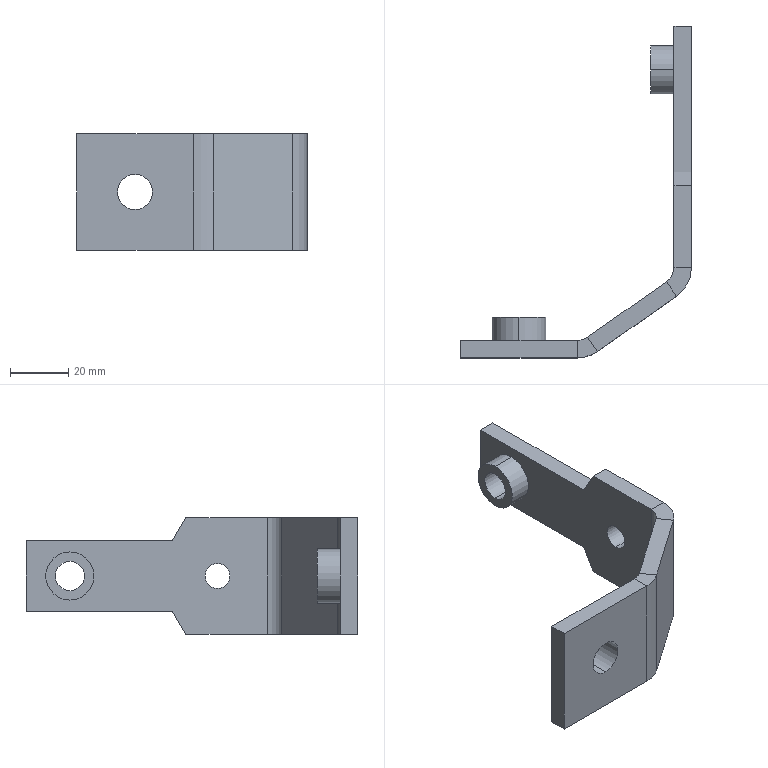Part | STEP file | 64586815 | 1 solid | 38 faces | box 79 x 113.5 x 40 mm | volume 36513 mm3 | plane 24 | cylinder 14 | commonest cylinder face diameters 12 x4 8.5 x2 10 x2 16.5 x2 18.5 x2 24 x2